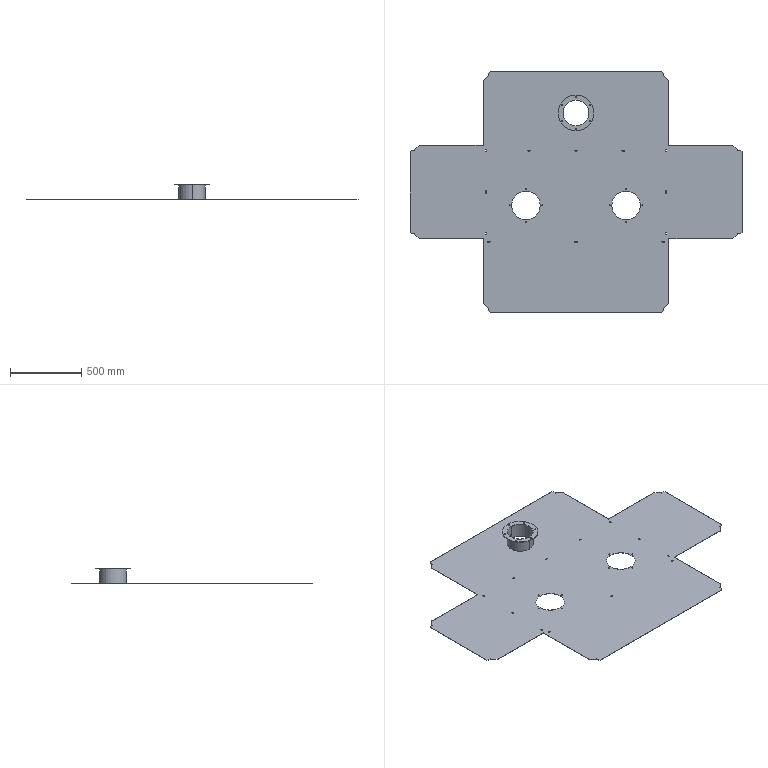Part | SolidWorks | features ICE 8, EdgeFlange 4, CirPattern 1, FlatPattern 1, SMBaseFlange 1, SheetMetal 1 | 1 solid | 169 faces | box 2323 x 1683 x 104.5 mm | volume 4309239 mm3 | plane 104 | cylinder 65 | commonest cylinder face diameters 7 x55 200 x4 180 x2 184 x2 250 x2